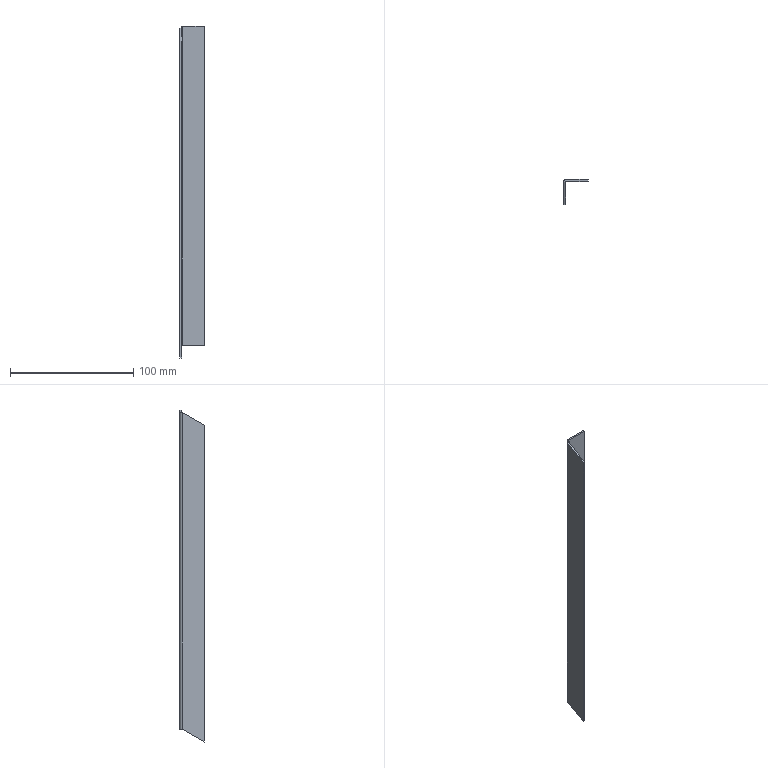Part | SolidWorks | features ICE 3, SMBaseFlange 2, EdgeFlange 1, FlatPattern 1, SheetMetal 1 | 1 solid | 18 faces | box 20 x 20 x 269.592 mm | volume 14701 mm3 | plane 16 | cylinder 2 | commonest cylinder face diameters 1 x1 4 x1
STEP:
#1=CARTESIAN_POINT('',(16.931,18.873,0.));
#2=VERTEX_POINT('',#1);
#3=CARTESIAN_POINT('',(16.931,18.873,257.2));
#4=VERTEX_POINT('',#3);
#5=CARTESIAN_POINT('',(16.931,18.873,0.));
#6=DIRECTION('',(0.,0.,1.));
#7=VECTOR('',#6,1000.);
#8=LINE('',#5,#7);
#9=EDGE_CURVE('',#2,#4,#8,.T.);
#10=ORIENTED_EDGE('',*,*,#9,.T.);
#11=CARTESIAN_POINT('',(17.431,18.873,257.2));
#12=VERTEX_POINT('',#11);
#13=CARTESIAN_POINT('',(8.688,18.873,257.2));
#14=DIRECTION('',(-1.,0.,0.));
#15=VECTOR('',#14,1000.);
#16=LINE('',#13,#15);
#17=EDGE_CURVE('',#12,#4,#16,.T.);
#18=ORIENTED_EDGE('',*,*,#17,.F.);
#19=CARTESIAN_POINT('',(17.431,18.873,257.7));
#20=VERTEX_POINT('',#19);
#21=CARTESIAN_POINT('',(17.431,18.873,257.7));
#22=DIRECTION('',(0.,0.,-1.));
#23=VECTOR('',#22,1000.);
#24=LINE('',#21,#23);
#25=EDGE_CURVE('',#20,#12,#24,.T.);
#26=ORIENTED_EDGE('',*,*,#25,.F.);
#27=CARTESIAN_POINT('',(16.431,18.873,257.7));
#28=VERTEX_POINT('',#27);
#29=CARTESIAN_POINT('',(8.688,18.873,257.7));
#30=DIRECTION('',(1.,0.,0.));
#31=VECTOR('',#30,1000.);
#32=LINE('',#29,#31);
#33=EDGE_CURVE('',#28,#20,#32,.T.);
#34=ORIENTED_EDGE('',*,*,#33,.F.);
#35=CARTESIAN_POINT('',(16.431,18.873,259.2));
#36=VERTEX_POINT('',#35);
#37=CARTESIAN_POINT('',(16.431,18.873,259.2));
#38=DIRECTION('',(0.,0.,-1.));
#39=VECTOR('',#38,1000.);
#40=LINE('',#37,#39);
#41=EDGE_CURVE('',#36,#28,#40,.T.);
#42=ORIENTED_EDGE('',*,*,#41,.F.);
#43=CARTESIAN_POINT('',(34.931,18.873,259.2));
#44=VERTEX_POINT('',#43);
#45=CARTESIAN_POINT('',(34.931,18.873,259.2));
#46=DIRECTION('',(-1.,0.,0.));
#47=VECTOR('',#46,1000.);
#48=LINE('',#45,#47);
#49=EDGE_CURVE('',#44,#36,#48,.T.);
#50=ORIENTED_EDGE('',*,*,#49,.F.);
#51=CARTESIAN_POINT('',(34.931,18.873,0.));
#52=VERTEX_POINT('',#51);
#53=CARTESIAN_POINT('',(34.931,18.873,259.2));
#54=DIRECTION('',(0.,0.,-1.));
#55=VECTOR('',#54,1000.);
#56=LINE('',#53,#55);
#57=EDGE_CURVE('',#44,#52,#56,.T.);
#58=ORIENTED_EDGE('',*,*,#57,.T.);
#59=CARTESIAN_POINT('',(34.931,18.873,0.));
#60=DIRECTION('',(-1.,0.,0.));
#61=VECTOR('',#60,1000.);
#62=LINE('',#59,#61);
#63=EDGE_CURVE('',#52,#2,#62,.T.);
#64=ORIENTED_EDGE('',*,*,#63,.T.);
#65=EDGE_LOOP('',(#10,#18,#26,#34,#42,#50,#58,#64));
#66=FACE_OUTER_BOUND('',#65,.T.);
#67=CARTESIAN_POINT('',(34.931,18.873,259.2));
#68=DIRECTION('',(0.,-1.,0.));
#69=DIRECTION('',(0.,0.,-1.));
#70=AXIS2_PLACEMENT_3D('',#67,#68,#69);
#71=PLANE('',#70);
#72=ADVANCED_FACE('',(#66),#71,.F.);
#73=CARTESIAN_POINT('',(16.931,17.373,257.2));
#74=VERTEX_POINT('',#73);
#75=CARTESIAN_POINT('',(17.431,17.373,257.2));
#76=VERTEX_POINT('',#75);
#77=CARTESIAN_POINT('',(34.931,17.373,257.2));
#78=DIRECTION('',(1.,0.,0.));
#79=VECTOR('',#78,1000.);
#80=LINE('',#77,#79);
#81=EDGE_CURVE('',#74,#76,#80,.T.);
#82=ORIENTED_EDGE('',*,*,#81,.F.);
#83=CARTESIAN_POINT('',(16.931,17.373,0.));
#84=VERTEX_POINT('',#83);
#85=CARTESIAN_POINT('',(16.931,17.373,0.));
#86=DIRECTION('',(0.,0.,1.));
#87=VECTOR('',#86,1000.);
#88=LINE('',#85,#87);
#89=EDGE_CURVE('',#84,#74,#88,.T.);
#90=ORIENTED_EDGE('',*,*,#89,.F.);
#91=CARTESIAN_POINT('',(34.931,17.373,0.));
#92=VERTEX_POINT('',#91);
#93=CARTESIAN_POINT('',(34.931,17.373,0.));
#94=DIRECTION('',(-1.,0.,0.));
#95=VECTOR('',#94,1000.);
#96=LINE('',#93,#95);
#97=EDGE_CURVE('',#92,#84,#96,.T.);
#98=ORIENTED_EDGE('',*,*,#97,.F.);
#99=CARTESIAN_POINT('',(34.931,17.373,259.2));
#100=VERTEX_POINT('',#99);
#101=CARTESIAN_POINT('',(34.931,17.373,259.2));
#102=DIRECTION('',(0.,0.,-1.));
#103=VECTOR('',#102,1000.);
#104=LINE('',#101,#103);
#105=EDGE_CURVE('',#100,#92,#104,.T.);
#106=ORIENTED_EDGE('',*,*,#105,.F.);
#107=CARTESIAN_POINT('',(16.431,17.373,259.2));
#108=VERTEX_POINT('',#107);
#109=CARTESIAN_POINT('',(34.931,17.373,259.2));
#110=DIRECTION('',(-1.,0.,0.));
#111=VECTOR('',#110,1000.);
#112=LINE('',#109,#111);
#113=EDGE_CURVE('',#100,#108,#112,.T.);
#114=ORIENTED_EDGE('',*,*,#113,.T.);
#115=CARTESIAN_POINT('',(16.431,17.373,257.7));
#116=VERTEX_POINT('',#115);
#117=CARTESIAN_POINT('',(16.431,17.373,259.2));
#118=DIRECTION('',(0.,0.,1.));
#119=VECTOR('',#118,1000.);
#120=LINE('',#117,#119);
#121=EDGE_CURVE('',#116,#108,#120,.T.);
#122=ORIENTED_EDGE('',*,*,#121,.F.);
#123=CARTESIAN_POINT('',(17.431,17.373,257.7));
#124=VERTEX_POINT('',#123);
#125=CARTESIAN_POINT('',(34.931,17.373,257.7));
#126=DIRECTION('',(-1.,0.,0.));
#127=VECTOR('',#126,1000.);
#128=LINE('',#125,#127);
#129=EDGE_CURVE('',#124,#116,#128,.T.);
#130=ORIENTED_EDGE('',*,*,#129,.F.);
#131=CARTESIAN_POINT('',(17.431,17.373,259.2));
#132=DIRECTION('',(0.,0.,1.));
#133=VECTOR('',#132,1000.);
#134=LINE('',#131,#133);
#135=EDGE_CURVE('',#76,#124,#134,.T.);
#136=ORIENTED_EDGE('',*,*,#135,.F.);
#137=EDGE_LOOP('',(#82,#90,#98,#106,#114,#122,#130,#136));
#138=FACE_OUTER_BOUND('',#137,.T.);
#139=CARTESIAN_POINT('',(34.931,17.373,259.2));
#140=DIRECTION('',(0.,-1.,0.));
#141=DIRECTION('',(0.,0.,-1.));
#142=AXIS2_PLACEMENT_3D('',#139,#140,#141);
#143=PLANE('',#142);
#144=ADVANCED_FACE('',(#138),#143,.T.);
#145=CARTESIAN_POINT('',(16.931,17.373,0.));
#146=DIRECTION('',(0.,1.,0.));
#147=VECTOR('',#146,1000.);
#148=LINE('',#145,#147);
#149=EDGE_CURVE('',#84,#2,#148,.T.);
#150=ORIENTED_EDGE('',*,*,#149,.T.);
#151=ORIENTED_EDGE('',*,*,#63,.F.);
#152=CARTESIAN_POINT('',(34.931,18.873,0.));
#153=DIRECTION('',(0.,-1.,0.));
#154=VECTOR('',#153,1000.);
#155=LINE('',#152,#154);
#156=EDGE_CURVE('',#52,#92,#155,.T.);
#157=ORIENTED_EDGE('',*,*,#156,.T.);
#158=ORIENTED_EDGE('',*,*,#97,.T.);
#159=EDGE_LOOP('',(#150,#151,#157,#158));
#160=FACE_OUTER_BOUND('',#159,.T.);
#161=CARTESIAN_POINT('',(0.,0.,0.));
#162=DIRECTION('',(0.,0.,1.));
#163=DIRECTION('',(1.,0.,0.));
#164=AXIS2_PLACEMENT_3D('',#161,#162,#163);
#165=PLANE('',#164);
#166=ADVANCED_FACE('',(#160),#165,.F.);
#167=CARTESIAN_POINT('',(16.931,17.373,257.2));
#168=DIRECTION('',(0.,1.,0.));
#169=VECTOR('',#168,1000.);
#170=LINE('',#167,#169);
#171=EDGE_CURVE('',#74,#4,#170,.T.);
#172=ORIENTED_EDGE('',*,*,#171,.F.);
#173=ORIENTED_EDGE('',*,*,#81,.T.);
#174=CARTESIAN_POINT('',(17.431,8.873,257.2));
#175=DIRECTION('',(0.,1.,0.));
#176=VECTOR('',#175,1000.);
#177=LINE('',#174,#176);
#178=EDGE_CURVE('',#76,#12,#177,.T.);
#179=ORIENTED_EDGE('',*,*,#178,.T.);
#180=ORIENTED_EDGE('',*,*,#17,.T.);
#181=EDGE_LOOP('',(#172,#173,#179,#180));
#182=FACE_OUTER_BOUND('',#181,.T.);
#183=CARTESIAN_POINT('',(8.688,8.873,257.2));
#184=DIRECTION('',(0.,0.,-1.));
#185=DIRECTION('',(-1.,0.,0.));
#186=AXIS2_PLACEMENT_3D('',#183,#184,#185);
#187=PLANE('',#186);
#188=ADVANCED_FACE('',(#182),#187,.F.);
#189=ORIENTED_EDGE('',*,*,#156,.F.);
#190=ORIENTED_EDGE('',*,*,#57,.F.);
#191=CARTESIAN_POINT('',(34.931,18.873,259.2));
#192=DIRECTION('',(0.,-1.,0.));
#193=VECTOR('',#192,1000.);
#194=LINE('',#191,#193);
#195=EDGE_CURVE('',#44,#100,#194,.T.);
#196=ORIENTED_EDGE('',*,*,#195,.T.);
#197=ORIENTED_EDGE('',*,*,#105,.T.);
#198=EDGE_LOOP('',(#189,#190,#196,#197));
#199=FACE_OUTER_BOUND('',#198,.T.);
#200=CARTESIAN_POINT('',(34.931,18.873,259.2));
#201=DIRECTION('',(1.,0.,0.));
#202=DIRECTION('',(0.,0.,-1.));
#203=AXIS2_PLACEMENT_3D('',#200,#201,#202);
#204=PLANE('',#203);
#205=ADVANCED_FACE('',(#199),#204,.T.);
#206=CARTESIAN_POINT('',(16.431,8.873,259.2));
#207=DIRECTION('',(0.,1.,0.));
#208=VECTOR('',#207,1000.);
#209=LINE('',#206,#208);
#210=EDGE_CURVE('',#108,#36,#209,.T.);
#211=ORIENTED_EDGE('',*,*,#210,.F.);
#212=ORIENTED_EDGE('',*,*,#113,.F.);
#213=ORIENTED_EDGE('',*,*,#195,.F.);
#214=ORIENTED_EDGE('',*,*,#49,.T.);
#215=EDGE_LOOP('',(#211,#212,#213,#214));
#216=FACE_OUTER_BOUND('',#215,.T.);
#217=CARTESIAN_POINT('',(0.,0.,259.2));
#218=DIRECTION('',(0.,0.,1.));
#219=DIRECTION('',(1.,0.,0.));
#220=AXIS2_PLACEMENT_3D('',#217,#218,#219);
#221=PLANE('',#220);
#222=ADVANCED_FACE('',(#216),#221,.T.);
#223=ORIENTED_EDGE('',*,*,#135,.T.);
#224=CARTESIAN_POINT('',(17.431,8.873,257.7));
#225=DIRECTION('',(0.,1.,0.));
#226=VECTOR('',#225,1000.);
#227=LINE('',#224,#226);
#228=EDGE_CURVE('',#124,#20,#227,.T.);
#229=ORIENTED_EDGE('',*,*,#228,.T.);
#230=ORIENTED_EDGE('',*,*,#25,.T.);
#231=ORIENTED_EDGE('',*,*,#178,.F.);
#232=EDGE_LOOP('',(#223,#229,#230,#231));
#233=FACE_OUTER_BOUND('',#232,.T.);
#234=CARTESIAN_POINT('',(17.431,8.873,257.7));
#235=DIRECTION('',(1.,0.,0.));
#236=DIRECTION('',(0.,0.,-1.));
#237=AXIS2_PLACEMENT_3D('',#234,#235,#236);
#238=PLANE('',#237);
#239=ADVANCED_FACE('',(#233),#238,.F.);
#240=ORIENTED_EDGE('',*,*,#129,.T.);
#241=CARTESIAN_POINT('',(16.431,8.873,257.7));
#242=DIRECTION('',(0.,1.,0.));
#243=VECTOR('',#242,1000.);
#244=LINE('',#241,#243);
#245=EDGE_CURVE('',#116,#28,#244,.T.);
#246=ORIENTED_EDGE('',*,*,#245,.T.);
#247=ORIENTED_EDGE('',*,*,#33,.T.);
#248=ORIENTED_EDGE('',*,*,#228,.F.);
#249=EDGE_LOOP('',(#240,#246,#247,#248));
#250=FACE_OUTER_BOUND('',#249,.T.);
#251=CARTESIAN_POINT('',(8.688,8.873,257.7));
#252=DIRECTION('',(0.,0.,1.));
#253=DIRECTION('',(1.,0.,0.));
#254=AXIS2_PLACEMENT_3D('',#251,#252,#253);
#255=PLANE('',#254);
#256=ADVANCED_FACE('',(#250),#255,.F.);
#257=ORIENTED_EDGE('',*,*,#121,.T.);
#258=ORIENTED_EDGE('',*,*,#210,.T.);
#259=ORIENTED_EDGE('',*,*,#41,.T.);
#260=ORIENTED_EDGE('',*,*,#245,.F.);
#261=EDGE_LOOP('',(#257,#258,#259,#260));
#262=FACE_OUTER_BOUND('',#261,.T.);
#263=CARTESIAN_POINT('',(16.431,8.873,259.2));
#264=DIRECTION('',(1.,0.,0.));
#265=DIRECTION('',(0.,0.,-1.));
#266=AXIS2_PLACEMENT_3D('',#263,#264,#265);
#267=PLANE('',#266);
#268=ADVANCED_FACE('',(#262),#267,.F.);
#269=CARTESIAN_POINT('',(16.431,16.873,257.2));
#270=VERTEX_POINT('',#269);
#271=CARTESIAN_POINT('',(14.931,16.873,257.2));
#272=VERTEX_POINT('',#271);
#273=CARTESIAN_POINT('',(14.931,16.873,257.2));
#274=DIRECTION('',(-1.,0.,0.));
#275=VECTOR('',#274,1000.);
#276=LINE('',#273,#275);
#277=EDGE_CURVE('',#270,#272,#276,.T.);
#278=ORIENTED_EDGE('',*,*,#277,.F.);
#279=CARTESIAN_POINT('',(16.931,16.873,257.2));
#280=DIRECTION('',(0.,0.,1.));
#281=DIRECTION('',(0.,1.,0.));
#282=AXIS2_PLACEMENT_3D('',#279,#280,#281);
#283=CIRCLE('',#282,0.5);
#284=EDGE_CURVE('',#74,#270,#283,.T.);
#285=ORIENTED_EDGE('',*,*,#284,.F.);
#286=ORIENTED_EDGE('',*,*,#171,.T.);
#287=CARTESIAN_POINT('',(16.931,16.873,257.2));
#288=DIRECTION('',(0.,0.,1.));
#289=DIRECTION('',(0.,1.,0.));
#290=AXIS2_PLACEMENT_3D('',#287,#288,#289);
#291=CIRCLE('',#290,2.);
#292=EDGE_CURVE('',#4,#272,#291,.T.);
#293=ORIENTED_EDGE('',*,*,#292,.T.);
#294=EDGE_LOOP('',(#278,#285,#286,#293));
#295=FACE_OUTER_BOUND('',#294,.T.);
#296=CARTESIAN_POINT('',(16.931,16.873,257.2));
#297=DIRECTION('',(0.,0.,1.));
#298=DIRECTION('',(0.,-1.,0.));
#299=AXIS2_PLACEMENT_3D('',#296,#297,#298);
#300=PLANE('',#299);
#301=ADVANCED_FACE('',(#295),#300,.T.);
#302=CARTESIAN_POINT('',(16.431,16.873,0.));
#303=VERTEX_POINT('',#302);
#304=CARTESIAN_POINT('',(16.931,16.873,0.));
#305=DIRECTION('',(0.,0.,-1.));
#306=DIRECTION('',(0.,1.,0.));
#307=AXIS2_PLACEMENT_3D('',#304,#305,#306);
#308=CIRCLE('',#307,0.5);
#309=EDGE_CURVE('',#303,#84,#308,.T.);
#310=ORIENTED_EDGE('',*,*,#309,.F.);
#311=CARTESIAN_POINT('',(14.931,16.873,0.));
#312=VERTEX_POINT('',#311);
#313=CARTESIAN_POINT('',(16.431,16.873,0.));
#314=DIRECTION('',(-1.,0.,0.));
#315=VECTOR('',#314,1000.);
#316=LINE('',#313,#315);
#317=EDGE_CURVE('',#303,#312,#316,.T.);
#318=ORIENTED_EDGE('',*,*,#317,.T.);
#319=CARTESIAN_POINT('',(16.931,16.873,0.));
#320=DIRECTION('',(0.,0.,-1.));
#321=DIRECTION('',(0.,1.,0.));
#322=AXIS2_PLACEMENT_3D('',#319,#320,#321);
#323=CIRCLE('',#322,2.);
#324=EDGE_CURVE('',#312,#2,#323,.T.);
#325=ORIENTED_EDGE('',*,*,#324,.T.);
#326=ORIENTED_EDGE('',*,*,#149,.F.);
#327=EDGE_LOOP('',(#310,#318,#325,#326));
#328=FACE_OUTER_BOUND('',#327,.T.);
#329=CARTESIAN_POINT('',(16.931,16.873,0.));
#330=DIRECTION('',(0.,0.,1.));
#331=DIRECTION('',(0.,-1.,0.));
#332=AXIS2_PLACEMENT_3D('',#329,#330,#331);
#333=PLANE('',#332);
#334=ADVANCED_FACE('',(#328),#333,.F.);
#335=ORIENTED_EDGE('',*,*,#9,.F.);
#336=ORIENTED_EDGE('',*,*,#324,.F.);
#337=CARTESIAN_POINT('',(14.931,16.873,0.));
#338=DIRECTION('',(0.,0.,-1.));
#339=VECTOR('',#338,1000.);
#340=LINE('',#337,#339);
#341=EDGE_CURVE('',#272,#312,#340,.T.);
#342=ORIENTED_EDGE('',*,*,#341,.F.);
#343=ORIENTED_EDGE('',*,*,#292,.F.);
#344=EDGE_LOOP('',(#335,#336,#342,#343));
#345=FACE_OUTER_BOUND('',#344,.T.);
#346=CARTESIAN_POINT('',(16.931,16.873,0.));
#347=DIRECTION('',(0.,0.,-1.));
#348=DIRECTION('',(-1.,0.,0.));
#349=AXIS2_PLACEMENT_3D('',#346,#347,#348);
#350=CYLINDRICAL_SURFACE('',#349,2.);
#351=ADVANCED_FACE('',(#345),#350,.T.);
#352=ORIENTED_EDGE('',*,*,#89,.T.);
#353=ORIENTED_EDGE('',*,*,#284,.T.);
#354=CARTESIAN_POINT('',(16.431,16.873,257.2));
#355=DIRECTION('',(0.,0.,-1.));
#356=VECTOR('',#355,1000.);
#357=LINE('',#354,#356);
#358=EDGE_CURVE('',#270,#303,#357,.T.);
#359=ORIENTED_EDGE('',*,*,#358,.T.);
#360=ORIENTED_EDGE('',*,*,#309,.T.);
#361=EDGE_LOOP('',(#352,#353,#359,#360));
#362=FACE_OUTER_BOUND('',#361,.T.);
#363=CARTESIAN_POINT('',(16.931,16.873,0.));
#364=DIRECTION('',(0.,0.,-1.));
#365=DIRECTION('',(-1.,0.,0.));
#366=AXIS2_PLACEMENT_3D('',#363,#364,#365);
#367=CYLINDRICAL_SURFACE('',#366,0.5);
#368=ADVANCED_FACE('',(#362),#367,.F.);
#369=CARTESIAN_POINT('',(14.931,-1.127,246.808));
#370=VERTEX_POINT('',#369);
#371=CARTESIAN_POINT('',(14.931,-107.153,185.594));
#372=DIRECTION('',(0.,-0.866,-0.5));
#373=VECTOR('',#372,1000.);
#374=LINE('',#371,#373);
#375=EDGE_CURVE('',#272,#370,#374,.T.);
#376=ORIENTED_EDGE('',*,*,#375,.F.);
#377=ORIENTED_EDGE('',*,*,#341,.T.);
#378=CARTESIAN_POINT('',(14.931,-1.127,-10.392));
#379=VERTEX_POINT('',#378);
#380=CARTESIAN_POINT('',(14.931,16.873,0.));
#381=DIRECTION('',(0.,0.866,0.5));
#382=VECTOR('',#381,1000.);
#383=LINE('',#380,#382);
#384=EDGE_CURVE('',#379,#312,#383,.T.);
#385=ORIENTED_EDGE('',*,*,#384,.F.);
#386=CARTESIAN_POINT('',(14.931,-1.127,0.));
#387=DIRECTION('',(0.,0.,-1.));
#388=VECTOR('',#387,1000.);
#389=LINE('',#386,#388);
#390=EDGE_CURVE('',#370,#379,#389,.T.);
#391=ORIENTED_EDGE('',*,*,#390,.F.);
#392=EDGE_LOOP('',(#376,#377,#385,#391));
#393=FACE_OUTER_BOUND('',#392,.T.);
#394=CARTESIAN_POINT('',(14.931,0.,0.));
#395=DIRECTION('',(-1.,0.,0.));
#396=DIRECTION('',(0.,-1.,0.));
#397=AXIS2_PLACEMENT_3D('',#394,#395,#396);
#398=PLANE('',#397);
#399=ADVANCED_FACE('',(#393),#398,.T.);
#400=ORIENTED_EDGE('',*,*,#358,.F.);
#401=CARTESIAN_POINT('',(16.431,-1.127,246.808));
#402=VERTEX_POINT('',#401);
#403=CARTESIAN_POINT('',(16.431,16.873,257.2));
#404=DIRECTION('',(0.,0.866,0.5));
#405=VECTOR('',#404,1000.);
#406=LINE('',#403,#405);
#407=EDGE_CURVE('',#402,#270,#406,.T.);
#408=ORIENTED_EDGE('',*,*,#407,.F.);
#409=CARTESIAN_POINT('',(16.431,-1.127,-10.392));
#410=VERTEX_POINT('',#409);
#411=CARTESIAN_POINT('',(16.431,-1.127,0.));
#412=DIRECTION('',(0.,0.,-1.));
#413=VECTOR('',#412,1000.);
#414=LINE('',#411,#413);
#415=EDGE_CURVE('',#402,#410,#414,.T.);
#416=ORIENTED_EDGE('',*,*,#415,.T.);
#417=CARTESIAN_POINT('',(16.431,16.873,0.));
#418=DIRECTION('',(0.,0.866,0.5));
#419=VECTOR('',#418,1000.);
#420=LINE('',#417,#419);
#421=EDGE_CURVE('',#410,#303,#420,.T.);
#422=ORIENTED_EDGE('',*,*,#421,.T.);
#423=EDGE_LOOP('',(#400,#408,#416,#422));
#424=FACE_OUTER_BOUND('',#423,.T.);
#425=CARTESIAN_POINT('',(16.431,0.,0.));
#426=DIRECTION('',(-1.,0.,0.));
#427=DIRECTION('',(0.,-1.,0.));
#428=AXIS2_PLACEMENT_3D('',#425,#426,#427);
#429=PLANE('',#428);
#430=ADVANCED_FACE('',(#424),#429,.F.);
#431=CARTESIAN_POINT('',(14.931,-1.127,246.808));
#432=DIRECTION('',(1.,0.,0.));
#433=VECTOR('',#432,1000.);
#434=LINE('',#431,#433);
#435=EDGE_CURVE('',#370,#402,#434,.T.);
#436=ORIENTED_EDGE('',*,*,#435,.F.);
#437=ORIENTED_EDGE('',*,*,#390,.T.);
#438=CARTESIAN_POINT('',(14.931,-1.127,-10.392));
#439=DIRECTION('',(1.,0.,0.));
#440=VECTOR('',#439,1000.);
#441=LINE('',#438,#440);
#442=EDGE_CURVE('',#379,#410,#441,.T.);
#443=ORIENTED_EDGE('',*,*,#442,.T.);
#444=ORIENTED_EDGE('',*,*,#415,.F.);
#445=EDGE_LOOP('',(#436,#437,#443,#444));
#446=FACE_OUTER_BOUND('',#445,.T.);
#447=CARTESIAN_POINT('',(14.931,-1.127,0.));
#448=DIRECTION('',(0.,-1.,0.));
#449=DIRECTION('',(1.,0.,0.));
#450=AXIS2_PLACEMENT_3D('',#447,#448,#449);
#451=PLANE('',#450);
#452=ADVANCED_FACE('',(#446),#451,.T.);
#453=ORIENTED_EDGE('',*,*,#375,.T.);
#454=ORIENTED_EDGE('',*,*,#435,.T.);
#455=ORIENTED_EDGE('',*,*,#407,.T.);
#456=ORIENTED_EDGE('',*,*,#277,.T.);
#457=EDGE_LOOP('',(#453,#454,#455,#456));
#458=FACE_OUTER_BOUND('',#457,.T.);
#459=CARTESIAN_POINT('',(6.431,16.873,257.2));
#460=DIRECTION('',(0.,0.5,-0.866));
#461=DIRECTION('',(0.,0.866,0.5));
#462=AXIS2_PLACEMENT_3D('',#459,#460,#461);
#463=PLANE('',#462);
#464=ADVANCED_FACE('',(#458),#463,.F.);
#465=ORIENTED_EDGE('',*,*,#421,.F.);
#466=ORIENTED_EDGE('',*,*,#442,.F.);
#467=ORIENTED_EDGE('',*,*,#384,.T.);
#468=ORIENTED_EDGE('',*,*,#317,.F.);
#469=EDGE_LOOP('',(#465,#466,#467,#468));
#470=FACE_OUTER_BOUND('',#469,.T.);
#471=CARTESIAN_POINT('',(14.931,16.873,0.));
#472=DIRECTION('',(0.,0.5,-0.866));
#473=DIRECTION('',(0.,0.866,0.5));
#474=AXIS2_PLACEMENT_3D('',#471,#472,#473);
#475=PLANE('',#474);
#476=ADVANCED_FACE('',(#470),#475,.T.);
#477=CLOSED_SHELL('',(#72,#144,#166,#188,#205,#222,#239,#256,#268,#301,#334,#351,#368,#399,#430,#452,#464,#476));
#478=MANIFOLD_SOLID_BREP('',#477);
#479=CARTESIAN_POINT('',(0.,0.,0.));
#480=DIRECTION('',(0.,0.,1.));
#481=DIRECTION('',(1.,0.,0.));
#482=AXIS2_PLACEMENT_3D('',#479,#480,#481);
#483=(LENGTH_UNIT()NAMED_UNIT(*)SI_UNIT(.MILLI.,.METRE.));
#484=UNCERTAINTY_MEASURE_WITH_UNIT(LENGTH_MEASURE(0.00001),#483,'','');
#485=(NAMED_UNIT(*)PLANE_ANGLE_UNIT()SI_UNIT($,.RADIAN.));
#486=(NAMED_UNIT(*)SI_UNIT($,.STERADIAN.)SOLID_ANGLE_UNIT());
#487=(GEOMETRIC_REPRESENTATION_CONTEXT(3)GLOBAL_UNCERTAINTY_ASSIGNED_CONTEXT((#484))GLOBAL_UNIT_ASSIGNED_CONTEXT((#483,#485,#486))REPRESENTATION_CONTEXT('',''));
#488=ADVANCED_BREP_SHAPE_REPRESENTATION('',(#478,#482),#487);